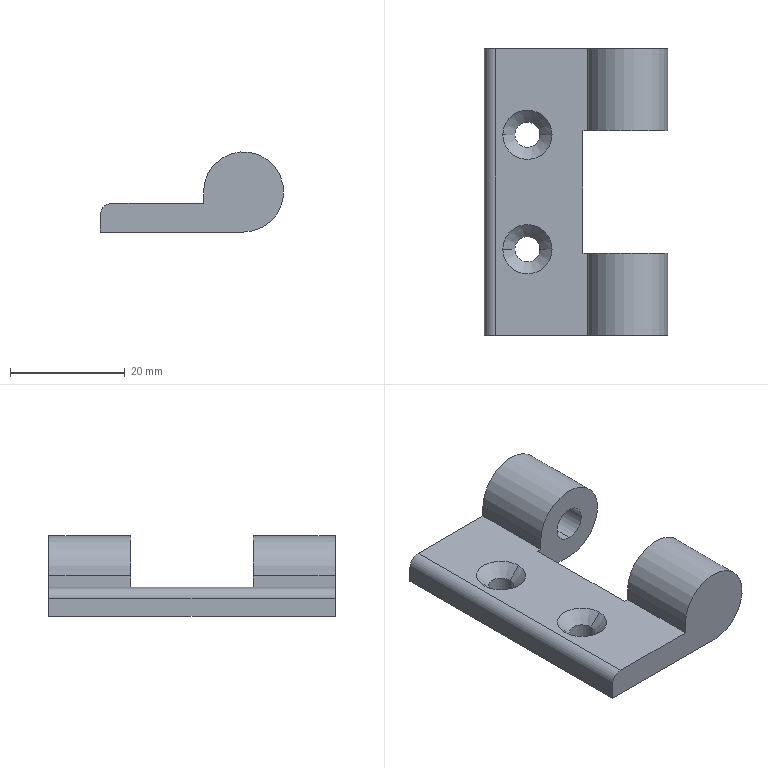Part | SolidWorks | features BaseBody 1 | 1 solid | 29 faces | box 32 x 50 x 14 mm | volume 8203 mm3 | cylinder 11 | plane 10 | sphere 4 | cone 4 | commonest cylinder face diameters 4.4 x4 6 x4 14 x2 4 x1
STEP:
#1=CARTESIAN_POINT('',(0.,-10.7,4.));
#2=VERTEX_POINT('',#1);
#3=CARTESIAN_POINT('',(0.,-10.7,10.));
#4=VERTEX_POINT('',#3);
#5=CARTESIAN_POINT('',(0.,-10.7,7.));
#6=DIRECTION('',(0.,-1.,0.));
#7=DIRECTION('',(0.,0.,1.));
#8=AXIS2_PLACEMENT_3D('',#5,#6,#7);
#9=CIRCLE('',#8,3.);
#10=EDGE_CURVE('',#2,#4,#9,.T.);
#11=ORIENTED_EDGE('',*,*,#10,.F.);
#12=CARTESIAN_POINT('',(0.,-20.,4.));
#13=VERTEX_POINT('',#12);
#14=CARTESIAN_POINT('',(0.,23.,4.));
#15=DIRECTION('',(0.,-1.,0.));
#16=VECTOR('',#15,1000.);
#17=LINE('',#14,#16);
#18=EDGE_CURVE('',#2,#13,#17,.T.);
#19=ORIENTED_EDGE('',*,*,#18,.T.);
#20=CARTESIAN_POINT('',(0.,-20.,10.));
#21=VERTEX_POINT('',#20);
#22=CARTESIAN_POINT('',(0.,-20.,7.));
#23=DIRECTION('',(0.,1.,0.));
#24=DIRECTION('',(0.,0.,1.));
#25=AXIS2_PLACEMENT_3D('',#22,#23,#24);
#26=CIRCLE('',#25,3.);
#27=EDGE_CURVE('',#21,#13,#26,.T.);
#28=ORIENTED_EDGE('',*,*,#27,.F.);
#29=CARTESIAN_POINT('',(0.,23.,10.));
#30=DIRECTION('',(0.,-1.,0.));
#31=VECTOR('',#30,1000.);
#32=LINE('',#29,#31);
#33=EDGE_CURVE('',#4,#21,#32,.T.);
#34=ORIENTED_EDGE('',*,*,#33,.F.);
#35=EDGE_LOOP('',(#11,#19,#28,#34));
#36=FACE_OUTER_BOUND('',#35,.T.);
#37=CARTESIAN_POINT('',(0.,23.,7.));
#38=DIRECTION('',(0.,-1.,0.));
#39=DIRECTION('',(0.,0.,1.));
#40=AXIS2_PLACEMENT_3D('',#37,#38,#39);
#41=CYLINDRICAL_SURFACE('',#40,3.);
#42=ADVANCED_FACE('',(#36),#41,.F.);
#43=CARTESIAN_POINT('',(0.,-23.,7.));
#44=VERTEX_POINT('',#43);
#45=CARTESIAN_POINT('',(0.,-20.,7.));
#46=DIRECTION('',(-1.,0.,0.));
#47=DIRECTION('',(0.,0.,1.));
#48=AXIS2_PLACEMENT_3D('',#45,#46,#47);
#49=CIRCLE('',#48,3.);
#50=EDGE_CURVE('',#44,#21,#49,.T.);
#51=ORIENTED_EDGE('',*,*,#50,.F.);
#52=CARTESIAN_POINT('',(0.,-20.,7.));
#53=DIRECTION('',(1.,0.,0.));
#54=DIRECTION('',(0.,0.,-1.));
#55=AXIS2_PLACEMENT_3D('',#52,#53,#54);
#56=CIRCLE('',#55,3.);
#57=EDGE_CURVE('',#44,#13,#56,.T.);
#58=ORIENTED_EDGE('',*,*,#57,.T.);
#59=CARTESIAN_POINT('',(0.,-20.,7.));
#60=DIRECTION('',(0.,1.,0.));
#61=DIRECTION('',(0.,0.,1.));
#62=AXIS2_PLACEMENT_3D('',#59,#60,#61);
#63=CIRCLE('',#62,3.);
#64=EDGE_CURVE('',#13,#21,#63,.T.);
#65=ORIENTED_EDGE('',*,*,#64,.T.);
#66=EDGE_LOOP('',(#51,#58,#65));
#67=FACE_OUTER_BOUND('',#66,.T.);
#68=CARTESIAN_POINT('',(0.,-20.,7.));
#69=DIRECTION('',(1.,0.,0.));
#70=DIRECTION('',(0.,0.,1.));
#71=AXIS2_PLACEMENT_3D('',#68,#69,#70);
#72=SPHERICAL_SURFACE('',#71,3.);
#73=ADVANCED_FACE('',(#67),#72,.F.);
#74=CARTESIAN_POINT('',(-15.3,-10.,2.9));
#75=VERTEX_POINT('',#74);
#76=CARTESIAN_POINT('',(-19.7,-10.,2.9));
#77=VERTEX_POINT('',#76);
#78=CARTESIAN_POINT('',(-17.5,-10.,2.9));
#79=DIRECTION('',(0.,0.,-1.));
#80=DIRECTION('',(-1.,0.,0.));
#81=AXIS2_PLACEMENT_3D('',#78,#79,#80);
#82=CIRCLE('',#81,2.2);
#83=EDGE_CURVE('',#75,#77,#82,.T.);
#84=ORIENTED_EDGE('',*,*,#83,.T.);
#85=CARTESIAN_POINT('',(-21.8,-10.,5.));
#86=VERTEX_POINT('',#85);
#87=CARTESIAN_POINT('',(-21.8,-10.,5.));
#88=DIRECTION('',(-0.7071,0.,0.7071));
#89=VECTOR('',#88,1000.);
#90=LINE('',#87,#89);
#91=EDGE_CURVE('',#77,#86,#90,.T.);
#92=ORIENTED_EDGE('',*,*,#91,.T.);
#93=CARTESIAN_POINT('',(-13.2,-10.,5.));
#94=VERTEX_POINT('',#93);
#95=CARTESIAN_POINT('',(-17.5,-10.,5.));
#96=DIRECTION('',(0.,0.,-1.));
#97=DIRECTION('',(-1.,0.,0.));
#98=AXIS2_PLACEMENT_3D('',#95,#96,#97);
#99=CIRCLE('',#98,4.3);
#100=EDGE_CURVE('',#94,#86,#99,.T.);
#101=ORIENTED_EDGE('',*,*,#100,.F.);
#102=CARTESIAN_POINT('',(-13.2,-10.,5.));
#103=DIRECTION('',(0.7071,0.,0.7071));
#104=VECTOR('',#103,1000.);
#105=LINE('',#102,#104);
#106=EDGE_CURVE('',#75,#94,#105,.T.);
#107=ORIENTED_EDGE('',*,*,#106,.F.);
#108=EDGE_LOOP('',(#84,#92,#101,#107));
#109=FACE_OUTER_BOUND('',#108,.T.);
#110=CARTESIAN_POINT('',(-17.5,-10.,5.));
#111=DIRECTION('',(0.,0.,1.));
#112=DIRECTION('',(1.,0.,0.));
#113=AXIS2_PLACEMENT_3D('',#110,#111,#112);
#114=CONICAL_SURFACE('',#113,4.3,0.7854);
#115=ADVANCED_FACE('',(#109),#114,.F.);
#116=CARTESIAN_POINT('',(-19.7,10.,0.));
#117=VERTEX_POINT('',#116);
#118=CARTESIAN_POINT('',(-15.3,10.,0.));
#119=VERTEX_POINT('',#118);
#120=CARTESIAN_POINT('',(-17.5,10.,0.));
#121=DIRECTION('',(0.,0.,-1.));
#122=DIRECTION('',(-1.,0.,0.));
#123=AXIS2_PLACEMENT_3D('',#120,#121,#122);
#124=CIRCLE('',#123,2.2);
#125=EDGE_CURVE('',#117,#119,#124,.T.);
#126=ORIENTED_EDGE('',*,*,#125,.T.);
#127=CARTESIAN_POINT('',(-15.3,10.,2.9));
#128=VERTEX_POINT('',#127);
#129=CARTESIAN_POINT('',(-15.3,10.,0.));
#130=DIRECTION('',(0.,0.,1.));
#131=VECTOR('',#130,1000.);
#132=LINE('',#129,#131);
#133=EDGE_CURVE('',#119,#128,#132,.T.);
#134=ORIENTED_EDGE('',*,*,#133,.T.);
#135=CARTESIAN_POINT('',(-19.7,10.,2.9));
#136=VERTEX_POINT('',#135);
#137=CARTESIAN_POINT('',(-17.5,10.,2.9));
#138=DIRECTION('',(0.,0.,-1.));
#139=DIRECTION('',(-1.,0.,0.));
#140=AXIS2_PLACEMENT_3D('',#137,#138,#139);
#141=CIRCLE('',#140,2.2);
#142=EDGE_CURVE('',#136,#128,#141,.T.);
#143=ORIENTED_EDGE('',*,*,#142,.F.);
#144=CARTESIAN_POINT('',(-19.7,10.,0.));
#145=DIRECTION('',(0.,0.,1.));
#146=VECTOR('',#145,1000.);
#147=LINE('',#144,#146);
#148=EDGE_CURVE('',#117,#136,#147,.T.);
#149=ORIENTED_EDGE('',*,*,#148,.F.);
#150=EDGE_LOOP('',(#126,#134,#143,#149));
#151=FACE_OUTER_BOUND('',#150,.T.);
#152=CARTESIAN_POINT('',(-17.5,10.,0.));
#153=DIRECTION('',(0.,0.,1.));
#154=DIRECTION('',(-1.,0.,0.));
#155=AXIS2_PLACEMENT_3D('',#152,#153,#154);
#156=CYLINDRICAL_SURFACE('',#155,2.2);
#157=ADVANCED_FACE('',(#151),#156,.F.);
#158=CARTESIAN_POINT('',(-17.5,10.,2.9));
#159=DIRECTION('',(0.,0.,-1.));
#160=DIRECTION('',(-1.,0.,0.));
#161=AXIS2_PLACEMENT_3D('',#158,#159,#160);
#162=CIRCLE('',#161,2.2);
#163=EDGE_CURVE('',#128,#136,#162,.T.);
#164=ORIENTED_EDGE('',*,*,#163,.T.);
#165=CARTESIAN_POINT('',(-21.8,10.,5.));
#166=VERTEX_POINT('',#165);
#167=CARTESIAN_POINT('',(-21.8,10.,5.));
#168=DIRECTION('',(-0.7071,0.,0.7071));
#169=VECTOR('',#168,1000.);
#170=LINE('',#167,#169);
#171=EDGE_CURVE('',#136,#166,#170,.T.);
#172=ORIENTED_EDGE('',*,*,#171,.T.);
#173=CARTESIAN_POINT('',(-13.2,10.,5.));
#174=VERTEX_POINT('',#173);
#175=CARTESIAN_POINT('',(-17.5,10.,5.));
#176=DIRECTION('',(0.,0.,-1.));
#177=DIRECTION('',(-1.,0.,0.));
#178=AXIS2_PLACEMENT_3D('',#175,#176,#177);
#179=CIRCLE('',#178,4.3);
#180=EDGE_CURVE('',#174,#166,#179,.T.);
#181=ORIENTED_EDGE('',*,*,#180,.F.);
#182=CARTESIAN_POINT('',(-13.2,10.,5.));
#183=DIRECTION('',(0.7071,0.,0.7071));
#184=VECTOR('',#183,1000.);
#185=LINE('',#182,#184);
#186=EDGE_CURVE('',#128,#174,#185,.T.);
#187=ORIENTED_EDGE('',*,*,#186,.F.);
#188=EDGE_LOOP('',(#164,#172,#181,#187));
#189=FACE_OUTER_BOUND('',#188,.T.);
#190=CARTESIAN_POINT('',(-17.5,10.,5.));
#191=DIRECTION('',(0.,0.,1.));
#192=DIRECTION('',(1.,0.,0.));
#193=AXIS2_PLACEMENT_3D('',#190,#191,#192);
#194=CONICAL_SURFACE('',#193,4.3,0.7854);
#195=ADVANCED_FACE('',(#189),#194,.F.);
#196=CARTESIAN_POINT('',(-19.7,-10.,0.));
#197=VERTEX_POINT('',#196);
#198=CARTESIAN_POINT('',(-15.3,-10.,0.));
#199=VERTEX_POINT('',#198);
#200=CARTESIAN_POINT('',(-17.5,-10.,0.));
#201=DIRECTION('',(0.,0.,-1.));
#202=DIRECTION('',(-1.,0.,0.));
#203=AXIS2_PLACEMENT_3D('',#200,#201,#202);
#204=CIRCLE('',#203,2.2);
#205=EDGE_CURVE('',#197,#199,#204,.T.);
#206=ORIENTED_EDGE('',*,*,#205,.T.);
#207=CARTESIAN_POINT('',(-15.3,-10.,0.));
#208=DIRECTION('',(0.,0.,1.));
#209=VECTOR('',#208,1000.);
#210=LINE('',#207,#209);
#211=EDGE_CURVE('',#199,#75,#210,.T.);
#212=ORIENTED_EDGE('',*,*,#211,.T.);
#213=CARTESIAN_POINT('',(-17.5,-10.,2.9));
#214=DIRECTION('',(0.,0.,-1.));
#215=DIRECTION('',(-1.,0.,0.));
#216=AXIS2_PLACEMENT_3D('',#213,#214,#215);
#217=CIRCLE('',#216,2.2);
#218=EDGE_CURVE('',#77,#75,#217,.T.);
#219=ORIENTED_EDGE('',*,*,#218,.F.);
#220=CARTESIAN_POINT('',(-19.7,-10.,0.));
#221=DIRECTION('',(0.,0.,1.));
#222=VECTOR('',#221,1000.);
#223=LINE('',#220,#222);
#224=EDGE_CURVE('',#197,#77,#223,.T.);
#225=ORIENTED_EDGE('',*,*,#224,.F.);
#226=EDGE_LOOP('',(#206,#212,#219,#225));
#227=FACE_OUTER_BOUND('',#226,.T.);
#228=CARTESIAN_POINT('',(-17.5,-10.,0.));
#229=DIRECTION('',(0.,0.,1.));
#230=DIRECTION('',(-1.,0.,0.));
#231=AXIS2_PLACEMENT_3D('',#228,#229,#230);
#232=CYLINDRICAL_SURFACE('',#231,2.2);
#233=ADVANCED_FACE('',(#227),#232,.F.);
#234=CARTESIAN_POINT('',(0.,20.,10.));
#235=VERTEX_POINT('',#234);
#236=CARTESIAN_POINT('',(0.,20.,4.));
#237=VERTEX_POINT('',#236);
#238=CARTESIAN_POINT('',(0.,20.,7.));
#239=DIRECTION('',(0.,1.,0.));
#240=DIRECTION('',(0.,0.,1.));
#241=AXIS2_PLACEMENT_3D('',#238,#239,#240);
#242=CIRCLE('',#241,3.);
#243=EDGE_CURVE('',#235,#237,#242,.T.);
#244=ORIENTED_EDGE('',*,*,#243,.T.);
#245=CARTESIAN_POINT('',(0.,10.7,4.));
#246=VERTEX_POINT('',#245);
#247=CARTESIAN_POINT('',(0.,23.,4.));
#248=DIRECTION('',(0.,-1.,0.));
#249=VECTOR('',#248,1000.);
#250=LINE('',#247,#249);
#251=EDGE_CURVE('',#237,#246,#250,.T.);
#252=ORIENTED_EDGE('',*,*,#251,.T.);
#253=CARTESIAN_POINT('',(0.,10.7,10.));
#254=VERTEX_POINT('',#253);
#255=CARTESIAN_POINT('',(0.,10.7,7.));
#256=DIRECTION('',(0.,1.,0.));
#257=DIRECTION('',(0.,0.,-1.));
#258=AXIS2_PLACEMENT_3D('',#255,#256,#257);
#259=CIRCLE('',#258,3.);
#260=EDGE_CURVE('',#254,#246,#259,.T.);
#261=ORIENTED_EDGE('',*,*,#260,.F.);
#262=CARTESIAN_POINT('',(0.,23.,10.));
#263=DIRECTION('',(0.,-1.,0.));
#264=VECTOR('',#263,1000.);
#265=LINE('',#262,#264);
#266=EDGE_CURVE('',#235,#254,#265,.T.);
#267=ORIENTED_EDGE('',*,*,#266,.F.);
#268=EDGE_LOOP('',(#244,#252,#261,#267));
#269=FACE_OUTER_BOUND('',#268,.T.);
#270=CARTESIAN_POINT('',(0.,23.,7.));
#271=DIRECTION('',(0.,-1.,0.));
#272=DIRECTION('',(0.,0.,1.));
#273=AXIS2_PLACEMENT_3D('',#270,#271,#272);
#274=CYLINDRICAL_SURFACE('',#273,3.);
#275=ADVANCED_FACE('',(#269),#274,.F.);
#276=ORIENTED_EDGE('',*,*,#243,.F.);
#277=CARTESIAN_POINT('',(0.,23.,7.));
#278=VERTEX_POINT('',#277);
#279=CARTESIAN_POINT('',(0.,20.,7.));
#280=DIRECTION('',(-1.,0.,0.));
#281=DIRECTION('',(0.,0.,1.));
#282=AXIS2_PLACEMENT_3D('',#279,#280,#281);
#283=CIRCLE('',#282,3.);
#284=EDGE_CURVE('',#235,#278,#283,.T.);
#285=ORIENTED_EDGE('',*,*,#284,.T.);
#286=CARTESIAN_POINT('',(0.,20.,7.));
#287=DIRECTION('',(1.,0.,0.));
#288=DIRECTION('',(0.,0.,-1.));
#289=AXIS2_PLACEMENT_3D('',#286,#287,#288);
#290=CIRCLE('',#289,3.);
#291=EDGE_CURVE('',#237,#278,#290,.T.);
#292=ORIENTED_EDGE('',*,*,#291,.F.);
#293=EDGE_LOOP('',(#276,#285,#292));
#294=FACE_OUTER_BOUND('',#293,.T.);
#295=CARTESIAN_POINT('',(0.,20.,7.));
#296=DIRECTION('',(-1.,0.,0.));
#297=DIRECTION('',(0.,0.,-1.));
#298=AXIS2_PLACEMENT_3D('',#295,#296,#297);
#299=SPHERICAL_SURFACE('',#298,3.);
#300=ADVANCED_FACE('',(#294),#299,.F.);
#301=ORIENTED_EDGE('',*,*,#284,.F.);
#302=CARTESIAN_POINT('',(0.,20.,7.));
#303=DIRECTION('',(0.,1.,0.));
#304=DIRECTION('',(0.,0.,1.));
#305=AXIS2_PLACEMENT_3D('',#302,#303,#304);
#306=CIRCLE('',#305,3.);
#307=EDGE_CURVE('',#237,#235,#306,.T.);
#308=ORIENTED_EDGE('',*,*,#307,.F.);
#309=ORIENTED_EDGE('',*,*,#291,.T.);
#310=EDGE_LOOP('',(#301,#308,#309));
#311=FACE_OUTER_BOUND('',#310,.T.);
#312=CARTESIAN_POINT('',(0.,20.,7.));
#313=DIRECTION('',(-1.,0.,0.));
#314=DIRECTION('',(0.,0.,-1.));
#315=AXIS2_PLACEMENT_3D('',#312,#313,#314);
#316=SPHERICAL_SURFACE('',#315,3.);
#317=ADVANCED_FACE('',(#311),#316,.F.);
#318=ORIENTED_EDGE('',*,*,#251,.F.);
#319=ORIENTED_EDGE('',*,*,#307,.T.);
#320=ORIENTED_EDGE('',*,*,#266,.T.);
#321=CARTESIAN_POINT('',(0.,10.7,7.));
#322=DIRECTION('',(0.,1.,0.));
#323=DIRECTION('',(0.,0.,-1.));
#324=AXIS2_PLACEMENT_3D('',#321,#322,#323);
#325=CIRCLE('',#324,3.);
#326=EDGE_CURVE('',#246,#254,#325,.T.);
#327=ORIENTED_EDGE('',*,*,#326,.F.);
#328=EDGE_LOOP('',(#318,#319,#320,#327));
#329=FACE_OUTER_BOUND('',#328,.T.);
#330=CARTESIAN_POINT('',(0.,23.,7.));
#331=DIRECTION('',(0.,-1.,0.));
#332=DIRECTION('',(0.,0.,1.));
#333=AXIS2_PLACEMENT_3D('',#330,#331,#332);
#334=CYLINDRICAL_SURFACE('',#333,3.);
#335=ADVANCED_FACE('',(#329),#334,.F.);
#336=ORIENTED_EDGE('',*,*,#211,.F.);
#337=CARTESIAN_POINT('',(-17.5,-10.,0.));
#338=DIRECTION('',(0.,0.,-1.));
#339=DIRECTION('',(-1.,0.,0.));
#340=AXIS2_PLACEMENT_3D('',#337,#338,#339);
#341=CIRCLE('',#340,2.2);
#342=EDGE_CURVE('',#199,#197,#341,.T.);
#343=ORIENTED_EDGE('',*,*,#342,.T.);
#344=ORIENTED_EDGE('',*,*,#224,.T.);
#345=ORIENTED_EDGE('',*,*,#83,.F.);
#346=EDGE_LOOP('',(#336,#343,#344,#345));
#347=FACE_OUTER_BOUND('',#346,.T.);
#348=CARTESIAN_POINT('',(-17.5,-10.,0.));
#349=DIRECTION('',(0.,0.,1.));
#350=DIRECTION('',(-1.,0.,0.));
#351=AXIS2_PLACEMENT_3D('',#348,#349,#350);
#352=CYLINDRICAL_SURFACE('',#351,2.2);
#353=ADVANCED_FACE('',(#347),#352,.F.);
#354=CARTESIAN_POINT('',(-7.8,-10.7,5.));
#355=VERTEX_POINT('',#354);
#356=CARTESIAN_POINT('',(-7.,-10.7,5.));
#357=VERTEX_POINT('',#356);
#358=CARTESIAN_POINT('',(-23.,-10.7,5.));
#359=DIRECTION('',(1.,0.,0.));
#360=VECTOR('',#359,1000.);
#361=LINE('',#358,#360);
#362=EDGE_CURVE('',#355,#357,#361,.T.);
#363=ORIENTED_EDGE('',*,*,#362,.F.);
#364=CARTESIAN_POINT('',(-7.8,10.7,5.));
#365=VERTEX_POINT('',#364);
#366=CARTESIAN_POINT('',(-7.8,25.,5.));
#367=DIRECTION('',(0.,-1.,0.));
#368=VECTOR('',#367,1000.);
#369=LINE('',#366,#368);
#370=EDGE_CURVE('',#365,#355,#369,.T.);
#371=ORIENTED_EDGE('',*,*,#370,.F.);
#372=CARTESIAN_POINT('',(-7.,10.7,5.));
#373=VERTEX_POINT('',#372);
#374=CARTESIAN_POINT('',(-23.,10.7,5.));
#375=DIRECTION('',(-1.,0.,0.));
#376=VECTOR('',#375,1000.);
#377=LINE('',#374,#376);
#378=EDGE_CURVE('',#373,#365,#377,.T.);
#379=ORIENTED_EDGE('',*,*,#378,.F.);
#380=CARTESIAN_POINT('',(-7.,25.,5.));
#381=VERTEX_POINT('',#380);
#382=CARTESIAN_POINT('',(-7.,25.,5.));
#383=DIRECTION('',(0.,-1.,0.));
#384=VECTOR('',#383,1000.);
#385=LINE('',#382,#384);
#386=EDGE_CURVE('',#381,#373,#385,.T.);
#387=ORIENTED_EDGE('',*,*,#386,.F.);
#388=CARTESIAN_POINT('',(-23.,25.,5.));
#389=VERTEX_POINT('',#388);
#390=CARTESIAN_POINT('',(-23.,25.,5.));
#391=DIRECTION('',(1.,0.,0.));
#392=VECTOR('',#391,1000.);
#393=LINE('',#390,#392);
#394=EDGE_CURVE('',#389,#381,#393,.T.);
#395=ORIENTED_EDGE('',*,*,#394,.F.);
#396=CARTESIAN_POINT('',(-23.,-25.,5.));
#397=VERTEX_POINT('',#396);
#398=CARTESIAN_POINT('',(-23.,25.,5.));
#399=DIRECTION('',(0.,-1.,0.));
#400=VECTOR('',#399,1000.);
#401=LINE('',#398,#400);
#402=EDGE_CURVE('',#389,#397,#401,.T.);
#403=ORIENTED_EDGE('',*,*,#402,.T.);
#404=CARTESIAN_POINT('',(-7.,-25.,5.));
#405=VERTEX_POINT('',#404);
#406=CARTESIAN_POINT('',(-23.,-25.,5.));
#407=DIRECTION('',(1.,0.,0.));
#408=VECTOR('',#407,1000.);
#409=LINE('',#406,#408);
#410=EDGE_CURVE('',#397,#405,#409,.T.);
#411=ORIENTED_EDGE('',*,*,#410,.T.);
#412=CARTESIAN_POINT('',(-7.,25.,5.));
#413=DIRECTION('',(0.,-1.,0.));
#414=VECTOR('',#413,1000.);
#415=LINE('',#412,#414);
#416=EDGE_CURVE('',#357,#405,#415,.T.);
#417=ORIENTED_EDGE('',*,*,#416,.F.);
#418=EDGE_LOOP('',(#363,#371,#379,#387,#395,#403,#411,#417));
#419=FACE_OUTER_BOUND('',#418,.T.);
#420=ORIENTED_EDGE('',*,*,#100,.T.);
#421=CARTESIAN_POINT('',(-17.5,-10.,5.));
#422=DIRECTION('',(0.,0.,-1.));
#423=DIRECTION('',(-1.,0.,0.));
#424=AXIS2_PLACEMENT_3D('',#421,#422,#423);
#425=CIRCLE('',#424,4.3);
#426=EDGE_CURVE('',#86,#94,#425,.T.);
#427=ORIENTED_EDGE('',*,*,#426,.T.);
#428=EDGE_LOOP('',(#420,#427));
#429=FACE_BOUND('',#428,.T.);
#430=ORIENTED_EDGE('',*,*,#180,.T.);
#431=CARTESIAN_POINT('',(-17.5,10.,5.));
#432=DIRECTION('',(0.,0.,-1.));
#433=DIRECTION('',(-1.,0.,0.));
#434=AXIS2_PLACEMENT_3D('',#431,#432,#433);
#435=CIRCLE('',#434,4.3);
#436=EDGE_CURVE('',#166,#174,#435,.T.);
#437=ORIENTED_EDGE('',*,*,#436,.T.);
#438=EDGE_LOOP('',(#430,#437));
#439=FACE_BOUND('',#438,.T.);
#440=CARTESIAN_POINT('',(-23.,25.,5.));
#441=DIRECTION('',(0.,0.,-1.));
#442=DIRECTION('',(0.,-1.,0.));
#443=AXIS2_PLACEMENT_3D('',#440,#441,#442);
#444=PLANE('',#443);
#445=ADVANCED_FACE('',(#419,#429,#439),#444,.F.);
#446=CARTESIAN_POINT('',(-7.,-10.7,7.));
#447=VERTEX_POINT('',#446);
#448=CARTESIAN_POINT('',(-7.,-10.7,5.));
#449=DIRECTION('',(0.,0.,1.));
#450=VECTOR('',#449,1000.);
#451=LINE('',#448,#450);
#452=EDGE_CURVE('',#357,#447,#451,.T.);
#453=ORIENTED_EDGE('',*,*,#452,.F.);
#454=ORIENTED_EDGE('',*,*,#416,.T.);
#455=CARTESIAN_POINT('',(-7.,-25.,7.));
#456=VERTEX_POINT('',#455);
#457=CARTESIAN_POINT('',(-7.,-25.,5.));
#458=DIRECTION('',(0.,0.,1.));
#459=VECTOR('',#458,1000.);
#460=LINE('',#457,#459);
#461=EDGE_CURVE('',#405,#456,#460,.T.);
#462=ORIENTED_EDGE('',*,*,#461,.T.);
#463=CARTESIAN_POINT('',(-7.,25.,7.));
#464=DIRECTION('',(0.,-1.,0.));
#465=VECTOR('',#464,1000.);
#466=LINE('',#463,#465);
#467=EDGE_CURVE('',#447,#456,#466,.T.);
#468=ORIENTED_EDGE('',*,*,#467,.F.);
#469=EDGE_LOOP('',(#453,#454,#462,#468));
#470=FACE_OUTER_BOUND('',#469,.T.);
#471=CARTESIAN_POINT('',(-7.,25.,5.));
#472=DIRECTION('',(1.,0.,0.));
#473=DIRECTION('',(0.,1.,0.));
#474=AXIS2_PLACEMENT_3D('',#471,#472,#473);
#475=PLANE('',#474);
#476=ADVANCED_FACE('',(#470),#475,.F.);
#477=CARTESIAN_POINT('',(-25.,-25.,3.));
#478=VERTEX_POINT('',#477);
#479=CARTESIAN_POINT('',(-23.,-25.,3.));
#480=DIRECTION('',(0.,1.,0.));
#481=DIRECTION('',(1.,0.,0.));
#482=AXIS2_PLACEMENT_3D('',#479,#480,#481);
#483=CIRCLE('',#482,2.);
#484=EDGE_CURVE('',#478,#397,#483,.T.);
#485=ORIENTED_EDGE('',*,*,#484,.T.);
#486=ORIENTED_EDGE('',*,*,#402,.F.);
#487=CARTESIAN_POINT('',(-25.,25.,3.));
#488=VERTEX_POINT('',#487);
#489=CARTESIAN_POINT('',(-23.,25.,3.));
#490=DIRECTION('',(0.,1.,0.));
#491=DIRECTION('',(1.,0.,0.));
#492=AXIS2_PLACEMENT_3D('',#489,#490,#491);
#493=CIRCLE('',#492,2.);
#494=EDGE_CURVE('',#488,#389,#493,.T.);
#495=ORIENTED_EDGE('',*,*,#494,.F.);
#496=CARTESIAN_POINT('',(-25.,25.,3.));
#497=DIRECTION('',(0.,-1.,0.));
#498=VECTOR('',#497,1000.);
#499=LINE('',#496,#498);
#500=EDGE_CURVE('',#488,#478,#499,.T.);
#501=ORIENTED_EDGE('',*,*,#500,.T.);
#502=EDGE_LOOP('',(#485,#486,#495,#501));
#503=FACE_OUTER_BOUND('',#502,.T.);
#504=CARTESIAN_POINT('',(-23.,25.,3.));
#505=DIRECTION('',(0.,1.,0.));
#506=DIRECTION('',(0.,0.,-1.));
#507=AXIS2_PLACEMENT_3D('',#504,#505,#506);
#508=CYLINDRICAL_SURFACE('',#507,2.);
#509=ADVANCED_FACE('',(#503),#508,.T.);
#510=CARTESIAN_POINT('',(-25.,25.,0.));
#511=VERTEX_POINT('',#510);
#512=CARTESIAN_POINT('',(-25.,25.,0.));
#513=DIRECTION('',(0.,0.,1.));
#514=VECTOR('',#513,1000.);
#515=LINE('',#512,#514);
#516=EDGE_CURVE('',#511,#488,#515,.T.);
#517=ORIENTED_EDGE('',*,*,#516,.T.);
#518=ORIENTED_EDGE('',*,*,#494,.T.);
#519=ORIENTED_EDGE('',*,*,#394,.T.);
#520=CARTESIAN_POINT('',(-7.,25.,7.));
#521=VERTEX_POINT('',#520);
#522=CARTESIAN_POINT('',(-7.,25.,5.));
#523=DIRECTION('',(0.,0.,1.));
#524=VECTOR('',#523,1000.);
#525=LINE('',#522,#524);
#526=EDGE_CURVE('',#381,#521,#525,.T.);
#527=ORIENTED_EDGE('',*,*,#526,.T.);
#528=CARTESIAN_POINT('',(0.,25.,0.));
#529=VERTEX_POINT('',#528);
#530=CARTESIAN_POINT('',(0.,25.,7.));
#531=DIRECTION('',(0.,1.,0.));
#532=DIRECTION('',(1.,0.,0.));
#533=AXIS2_PLACEMENT_3D('',#530,#531,#532);
#534=CIRCLE('',#533,7.);
#535=EDGE_CURVE('',#521,#529,#534,.T.);
#536=ORIENTED_EDGE('',*,*,#535,.T.);
#537=CARTESIAN_POINT('',(0.,25.,0.));
#538=DIRECTION('',(-1.,0.,0.));
#539=VECTOR('',#538,1000.);
#540=LINE('',#537,#539);
#541=EDGE_CURVE('',#529,#511,#540,.T.);
#542=ORIENTED_EDGE('',*,*,#541,.T.);
#543=EDGE_LOOP('',(#517,#518,#519,#527,#536,#542));
#544=FACE_OUTER_BOUND('',#543,.T.);
#545=CARTESIAN_POINT('',(-23.,25.,3.));
#546=DIRECTION('',(0.,1.,0.));
#547=DIRECTION('',(1.,0.,0.));
#548=AXIS2_PLACEMENT_3D('',#545,#546,#547);
#549=PLANE('',#548);
#550=ADVANCED_FACE('',(#544),#549,.T.);
#551=CARTESIAN_POINT('',(-25.,-25.,0.));
#552=VERTEX_POINT('',#551);
#553=CARTESIAN_POINT('',(-25.,-25.,0.));
#554=DIRECTION('',(0.,0.,1.));
#555=VECTOR('',#554,1000.);
#556=LINE('',#553,#555);
#557=EDGE_CURVE('',#552,#478,#556,.T.);
#558=ORIENTED_EDGE('',*,*,#557,.T.);
#559=ORIENTED_EDGE('',*,*,#500,.F.);
#560=ORIENTED_EDGE('',*,*,#516,.F.);
#561=CARTESIAN_POINT('',(-25.,25.,0.));
#562=DIRECTION('',(0.,-1.,0.));
#563=VECTOR('',#562,1000.);
#564=LINE('',#561,#563);
#565=EDGE_CURVE('',#511,#552,#564,.T.);
#566=ORIENTED_EDGE('',*,*,#565,.T.);
#567=EDGE_LOOP('',(#558,#559,#560,#566));
#568=FACE_OUTER_BOUND('',#567,.T.);
#569=CARTESIAN_POINT('',(-25.,25.,0.));
#570=DIRECTION('',(1.,0.,0.));
#571=DIRECTION('',(0.,1.,0.));
#572=AXIS2_PLACEMENT_3D('',#569,#570,#571);
#573=PLANE('',#572);
#574=ADVANCED_FACE('',(#568),#573,.F.);
#575=CARTESIAN_POINT('',(-7.8,-10.7,0.));
#576=VERTEX_POINT('',#575);
#577=CARTESIAN_POINT('',(0.,-10.7,0.));
#578=VERTEX_POINT('',#577);
#579=CARTESIAN_POINT('',(-7.8,-10.7,0.));
#580=DIRECTION('',(1.,0.,0.));
#581=VECTOR('',#580,1000.);
#582=LINE('',#579,#581);
#583=EDGE_CURVE('',#576,#578,#582,.T.);
#584=ORIENTED_EDGE('',*,*,#583,.T.);
#585=CARTESIAN_POINT('',(0.,-25.,0.));
#586=VERTEX_POINT('',#585);
#587=CARTESIAN_POINT('',(0.,25.,0.));
#588=DIRECTION('',(0.,-1.,0.));
#589=VECTOR('',#588,1000.);
#590=LINE('',#587,#589);
#591=EDGE_CURVE('',#578,#586,#590,.T.);
#592=ORIENTED_EDGE('',*,*,#591,.T.);
#593=CARTESIAN_POINT('',(0.,-25.,0.));
#594=DIRECTION('',(-1.,0.,0.));
#595=VECTOR('',#594,1000.);
#596=LINE('',#593,#595);
#597=EDGE_CURVE('',#586,#552,#596,.T.);
#598=ORIENTED_EDGE('',*,*,#597,.T.);
#599=ORIENTED_EDGE('',*,*,#565,.F.);
#600=ORIENTED_EDGE('',*,*,#541,.F.);
#601=CARTESIAN_POINT('',(0.,10.7,0.));
#602=VERTEX_POINT('',#601);
#603=CARTESIAN_POINT('',(0.,25.,0.));
#604=DIRECTION('',(0.,-1.,0.));
#605=VECTOR('',#604,1000.);
#606=LINE('',#603,#605);
#607=EDGE_CURVE('',#529,#602,#606,.T.);
#608=ORIENTED_EDGE('',*,*,#607,.T.);
#609=CARTESIAN_POINT('',(-7.8,10.7,0.));
#610=VERTEX_POINT('',#609);
#611=CARTESIAN_POINT('',(7.,10.7,0.));
#612=DIRECTION('',(-1.,0.,0.));
#613=VECTOR('',#612,1000.);
#614=LINE('',#611,#613);
#615=EDGE_CURVE('',#602,#610,#614,.T.);
#616=ORIENTED_EDGE('',*,*,#615,.T.);
#617=CARTESIAN_POINT('',(-7.8,10.7,0.));
#618=DIRECTION('',(0.,-1.,0.));
#619=VECTOR('',#618,1000.);
#620=LINE('',#617,#619);
#621=EDGE_CURVE('',#610,#576,#620,.T.);
#622=ORIENTED_EDGE('',*,*,#621,.T.);
#623=EDGE_LOOP('',(#584,#592,#598,#599,#600,#608,#616,#622));
#624=FACE_OUTER_BOUND('',#623,.T.);
#625=ORIENTED_EDGE('',*,*,#205,.F.);
#626=ORIENTED_EDGE('',*,*,#342,.F.);
#627=EDGE_LOOP('',(#625,#626));
#628=FACE_BOUND('',#627,.T.);
#629=ORIENTED_EDGE('',*,*,#125,.F.);
#630=CARTESIAN_POINT('',(-17.5,10.,0.));
#631=DIRECTION('',(0.,0.,-1.));
#632=DIRECTION('',(-1.,0.,0.));
#633=AXIS2_PLACEMENT_3D('',#630,#631,#632);
#634=CIRCLE('',#633,2.2);
#635=EDGE_CURVE('',#119,#117,#634,.T.);
#636=ORIENTED_EDGE('',*,*,#635,.F.);
#637=EDGE_LOOP('',(#629,#636));
#638=FACE_BOUND('',#637,.T.);
#639=CARTESIAN_POINT('',(0.,25.,0.));
#640=DIRECTION('',(0.,0.,1.));
#641=DIRECTION('',(1.,0.,0.));
#642=AXIS2_PLACEMENT_3D('',#639,#640,#641);
#643=PLANE('',#642);
#644=ADVANCED_FACE('',(#624,#628,#638),#643,.F.);
#645=CARTESIAN_POINT('',(-7.,10.7,7.));
#646=VERTEX_POINT('',#645);
#647=CARTESIAN_POINT('',(0.,10.7,7.));
#648=DIRECTION('',(0.,-1.,0.));
#649=DIRECTION('',(0.,0.,-1.));
#650=AXIS2_PLACEMENT_3D('',#647,#648,#649);
#651=CIRCLE('',#650,7.);
#652=EDGE_CURVE('',#602,#646,#651,.T.);
#653=ORIENTED_EDGE('',*,*,#652,.F.);
#654=ORIENTED_EDGE('',*,*,#607,.F.);
#655=ORIENTED_EDGE('',*,*,#535,.F.);
#656=CARTESIAN_POINT('',(-7.,25.,7.));
#657=DIRECTION('',(0.,-1.,0.));
#658=VECTOR('',#657,1000.);
#659=LINE('',#656,#658);
#660=EDGE_CURVE('',#521,#646,#659,.T.);
#661=ORIENTED_EDGE('',*,*,#660,.T.);
#662=EDGE_LOOP('',(#653,#654,#655,#661));
#663=FACE_OUTER_BOUND('',#662,.T.);
#664=CARTESIAN_POINT('',(0.,25.,7.));
#665=DIRECTION('',(0.,1.,0.));
#666=DIRECTION('',(0.,0.,-1.));
#667=AXIS2_PLACEMENT_3D('',#664,#665,#666);
#668=CYLINDRICAL_SURFACE('',#667,7.);
#669=ADVANCED_FACE('',(#663),#668,.T.);
#670=CARTESIAN_POINT('',(0.,-10.7,7.));
#671=DIRECTION('',(0.,1.,0.));
#672=DIRECTION('',(0.,0.,1.));
#673=AXIS2_PLACEMENT_3D('',#670,#671,#672);
#674=CIRCLE('',#673,7.);
#675=EDGE_CURVE('',#447,#578,#674,.T.);
#676=ORIENTED_EDGE('',*,*,#675,.F.);
#677=ORIENTED_EDGE('',*,*,#467,.T.);
#678=CARTESIAN_POINT('',(0.,-25.,7.));
#679=DIRECTION('',(0.,1.,0.));
#680=DIRECTION('',(1.,0.,0.));
#681=AXIS2_PLACEMENT_3D('',#678,#679,#680);
#682=CIRCLE('',#681,7.);
#683=EDGE_CURVE('',#456,#586,#682,.T.);
#684=ORIENTED_EDGE('',*,*,#683,.T.);
#685=ORIENTED_EDGE('',*,*,#591,.F.);
#686=EDGE_LOOP('',(#676,#677,#684,#685));
#687=FACE_OUTER_BOUND('',#686,.T.);
#688=CARTESIAN_POINT('',(0.,25.,7.));
#689=DIRECTION('',(0.,1.,0.));
#690=DIRECTION('',(0.,0.,-1.));
#691=AXIS2_PLACEMENT_3D('',#688,#689,#690);
#692=CYLINDRICAL_SURFACE('',#691,7.);
#693=ADVANCED_FACE('',(#687),#692,.T.);
#694=CARTESIAN_POINT('',(-7.,10.7,5.));
#695=DIRECTION('',(0.,0.,-1.));
#696=VECTOR('',#695,1000.);
#697=LINE('',#694,#696);
#698=EDGE_CURVE('',#646,#373,#697,.T.);
#699=ORIENTED_EDGE('',*,*,#698,.F.);
#700=ORIENTED_EDGE('',*,*,#660,.F.);
#701=ORIENTED_EDGE('',*,*,#526,.F.);
#702=ORIENTED_EDGE('',*,*,#386,.T.);
#703=EDGE_LOOP('',(#699,#700,#701,#702));
#704=FACE_OUTER_BOUND('',#703,.T.);
#705=CARTESIAN_POINT('',(-7.,25.,5.));
#706=DIRECTION('',(1.,0.,0.));
#707=DIRECTION('',(0.,1.,0.));
#708=AXIS2_PLACEMENT_3D('',#705,#706,#707);
#709=PLANE('',#708);
#710=ADVANCED_FACE('',(#704),#709,.F.);
#711=ORIENTED_EDGE('',*,*,#378,.T.);
#712=CARTESIAN_POINT('',(-7.8,10.7,14.));
#713=DIRECTION('',(0.,0.,-1.));
#714=VECTOR('',#713,1000.);
#715=LINE('',#712,#714);
#716=EDGE_CURVE('',#365,#610,#715,.T.);
#717=ORIENTED_EDGE('',*,*,#716,.T.);
#718=ORIENTED_EDGE('',*,*,#615,.F.);
#719=ORIENTED_EDGE('',*,*,#652,.T.);
#720=ORIENTED_EDGE('',*,*,#698,.T.);
#721=EDGE_LOOP('',(#711,#717,#718,#719,#720));
#722=FACE_OUTER_BOUND('',#721,.T.);
#723=ORIENTED_EDGE('',*,*,#260,.T.);
#724=ORIENTED_EDGE('',*,*,#326,.T.);
#725=EDGE_LOOP('',(#723,#724));
#726=FACE_BOUND('',#725,.T.);
#727=CARTESIAN_POINT('',(7.,10.7,14.));
#728=DIRECTION('',(0.,-1.,0.));
#729=DIRECTION('',(0.,0.,-1.));
#730=AXIS2_PLACEMENT_3D('',#727,#728,#729);
#731=PLANE('',#730);
#732=ADVANCED_FACE('',(#722,#726),#731,.T.);
#733=ORIENTED_EDGE('',*,*,#171,.F.);
#734=ORIENTED_EDGE('',*,*,#142,.T.);
#735=ORIENTED_EDGE('',*,*,#186,.T.);
#736=ORIENTED_EDGE('',*,*,#436,.F.);
#737=EDGE_LOOP('',(#733,#734,#735,#736));
#738=FACE_OUTER_BOUND('',#737,.T.);
#739=CARTESIAN_POINT('',(-17.5,10.,5.));
#740=DIRECTION('',(0.,0.,1.));
#741=DIRECTION('',(1.,0.,0.));
#742=AXIS2_PLACEMENT_3D('',#739,#740,#741);
#743=CONICAL_SURFACE('',#742,4.3,0.7854);
#744=ADVANCED_FACE('',(#738),#743,.F.);
#745=ORIENTED_EDGE('',*,*,#675,.T.);
#746=ORIENTED_EDGE('',*,*,#583,.F.);
#747=CARTESIAN_POINT('',(-7.8,-10.7,14.));
#748=DIRECTION('',(0.,0.,-1.));
#749=VECTOR('',#748,1000.);
#750=LINE('',#747,#749);
#751=EDGE_CURVE('',#355,#576,#750,.T.);
#752=ORIENTED_EDGE('',*,*,#751,.F.);
#753=ORIENTED_EDGE('',*,*,#362,.T.);
#754=ORIENTED_EDGE('',*,*,#452,.T.);
#755=EDGE_LOOP('',(#745,#746,#752,#753,#754));
#756=FACE_OUTER_BOUND('',#755,.T.);
#757=CARTESIAN_POINT('',(0.,-10.7,7.));
#758=DIRECTION('',(0.,-1.,0.));
#759=DIRECTION('',(0.,0.,1.));
#760=AXIS2_PLACEMENT_3D('',#757,#758,#759);
#761=CIRCLE('',#760,3.);
#762=EDGE_CURVE('',#4,#2,#761,.T.);
#763=ORIENTED_EDGE('',*,*,#762,.T.);
#764=ORIENTED_EDGE('',*,*,#10,.T.);
#765=EDGE_LOOP('',(#763,#764));
#766=FACE_BOUND('',#765,.T.);
#767=CARTESIAN_POINT('',(-7.8,-10.7,14.));
#768=DIRECTION('',(0.,1.,0.));
#769=DIRECTION('',(1.,0.,0.));
#770=AXIS2_PLACEMENT_3D('',#767,#768,#769);
#771=PLANE('',#770);
#772=ADVANCED_FACE('',(#756,#766),#771,.T.);
#773=ORIENTED_EDGE('',*,*,#370,.T.);
#774=ORIENTED_EDGE('',*,*,#751,.T.);
#775=ORIENTED_EDGE('',*,*,#621,.F.);
#776=ORIENTED_EDGE('',*,*,#716,.F.);
#777=EDGE_LOOP('',(#773,#774,#775,#776));
#778=FACE_OUTER_BOUND('',#777,.T.);
#779=CARTESIAN_POINT('',(-7.8,10.7,14.));
#780=DIRECTION('',(1.,0.,0.));
#781=DIRECTION('',(0.,1.,0.));
#782=AXIS2_PLACEMENT_3D('',#779,#780,#781);
#783=PLANE('',#782);
#784=ADVANCED_FACE('',(#778),#783,.T.);
#785=ORIENTED_EDGE('',*,*,#557,.F.);
#786=ORIENTED_EDGE('',*,*,#597,.F.);
#787=ORIENTED_EDGE('',*,*,#683,.F.);
#788=ORIENTED_EDGE('',*,*,#461,.F.);
#789=ORIENTED_EDGE('',*,*,#410,.F.);
#790=ORIENTED_EDGE('',*,*,#484,.F.);
#791=EDGE_LOOP('',(#785,#786,#787,#788,#789,#790));
#792=FACE_OUTER_BOUND('',#791,.T.);
#793=CARTESIAN_POINT('',(-23.,-25.,3.));
#794=DIRECTION('',(0.,1.,0.));
#795=DIRECTION('',(1.,0.,0.));
#796=AXIS2_PLACEMENT_3D('',#793,#794,#795);
#797=PLANE('',#796);
#798=ADVANCED_FACE('',(#792),#797,.F.);
#799=ORIENTED_EDGE('',*,*,#133,.F.);
#800=ORIENTED_EDGE('',*,*,#635,.T.);
#801=ORIENTED_EDGE('',*,*,#148,.T.);
#802=ORIENTED_EDGE('',*,*,#163,.F.);
#803=EDGE_LOOP('',(#799,#800,#801,#802));
#804=FACE_OUTER_BOUND('',#803,.T.);
#805=CARTESIAN_POINT('',(-17.5,10.,0.));
#806=DIRECTION('',(0.,0.,1.));
#807=DIRECTION('',(-1.,0.,0.));
#808=AXIS2_PLACEMENT_3D('',#805,#806,#807);
#809=CYLINDRICAL_SURFACE('',#808,2.2);
#810=ADVANCED_FACE('',(#804),#809,.F.);
#811=ORIENTED_EDGE('',*,*,#91,.F.);
#812=ORIENTED_EDGE('',*,*,#218,.T.);
#813=ORIENTED_EDGE('',*,*,#106,.T.);
#814=ORIENTED_EDGE('',*,*,#426,.F.);
#815=EDGE_LOOP('',(#811,#812,#813,#814));
#816=FACE_OUTER_BOUND('',#815,.T.);
#817=CARTESIAN_POINT('',(-17.5,-10.,5.));
#818=DIRECTION('',(0.,0.,1.));
#819=DIRECTION('',(1.,0.,0.));
#820=AXIS2_PLACEMENT_3D('',#817,#818,#819);
#821=CONICAL_SURFACE('',#820,4.3,0.7854);
#822=ADVANCED_FACE('',(#816),#821,.F.);
#823=ORIENTED_EDGE('',*,*,#57,.F.);
#824=ORIENTED_EDGE('',*,*,#50,.T.);
#825=ORIENTED_EDGE('',*,*,#27,.T.);
#826=EDGE_LOOP('',(#823,#824,#825));
#827=FACE_OUTER_BOUND('',#826,.T.);
#828=CARTESIAN_POINT('',(0.,-20.,7.));
#829=DIRECTION('',(1.,0.,0.));
#830=DIRECTION('',(0.,0.,1.));
#831=AXIS2_PLACEMENT_3D('',#828,#829,#830);
#832=SPHERICAL_SURFACE('',#831,3.);
#833=ADVANCED_FACE('',(#827),#832,.F.);
#834=ORIENTED_EDGE('',*,*,#18,.F.);
#835=ORIENTED_EDGE('',*,*,#762,.F.);
#836=ORIENTED_EDGE('',*,*,#33,.T.);
#837=ORIENTED_EDGE('',*,*,#64,.F.);
#838=EDGE_LOOP('',(#834,#835,#836,#837));
#839=FACE_OUTER_BOUND('',#838,.T.);
#840=CARTESIAN_POINT('',(0.,23.,7.));
#841=DIRECTION('',(0.,-1.,0.));
#842=DIRECTION('',(0.,0.,1.));
#843=AXIS2_PLACEMENT_3D('',#840,#841,#842);
#844=CYLINDRICAL_SURFACE('',#843,3.);
#845=ADVANCED_FACE('',(#839),#844,.F.);
#846=CLOSED_SHELL('',(#42,#73,#115,#157,#195,#233,#275,#300,#317,#335,#353,#445,#476,#509,#550,#574,#644,#669,#693,#710,#732,#744,#772,#784,#798,#810,#822,#833,#845));
#847=MANIFOLD_SOLID_BREP('',#846);
#848=CARTESIAN_POINT('',(0.,0.,0.));
#849=DIRECTION('',(0.,0.,1.));
#850=DIRECTION('',(1.,0.,0.));
#851=AXIS2_PLACEMENT_3D('',#848,#849,#850);
#852=(LENGTH_UNIT()NAMED_UNIT(*)SI_UNIT(.MILLI.,.METRE.));
#853=UNCERTAINTY_MEASURE_WITH_UNIT(LENGTH_MEASURE(0.00001),#852,'','');
#854=(NAMED_UNIT(*)PLANE_ANGLE_UNIT()SI_UNIT($,.RADIAN.));
#855=(NAMED_UNIT(*)SI_UNIT($,.STERADIAN.)SOLID_ANGLE_UNIT());
#856=(GEOMETRIC_REPRESENTATION_CONTEXT(3)GLOBAL_UNCERTAINTY_ASSIGNED_CONTEXT((#853))GLOBAL_UNIT_ASSIGNED_CONTEXT((#852,#854,#855))REPRESENTATION_CONTEXT('',''));
#857=ADVANCED_BREP_SHAPE_REPRESENTATION('',(#847,#851),#856);